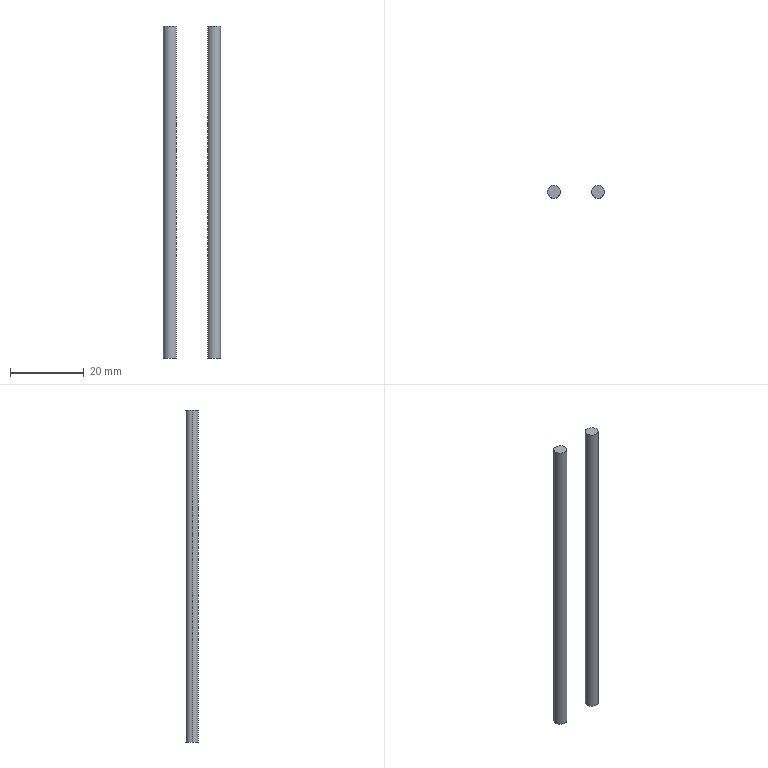Part | SolidWorks | features BaseBody 2 | 2 solids | 8 faces | box 15.5 x 3.5 x 90 mm | volume 1732 mm3 | plane 4 | cylinder 4 | commonest cylinder face diameters 3.5 x4
STEP:
#1=CARTESIAN_POINT('',(-1.75,0.,0.));
#2=VERTEX_POINT('',#1);
#3=CARTESIAN_POINT('',(1.75,0.,0.));
#4=VERTEX_POINT('',#3);
#5=CARTESIAN_POINT('',(0.,0.,0.));
#6=DIRECTION('',(0.,0.,1.));
#7=DIRECTION('',(1.,0.,0.));
#8=AXIS2_PLACEMENT_3D('',#5,#6,#7);
#9=CIRCLE('',#8,1.75);
#10=EDGE_CURVE('',#2,#4,#9,.T.);
#11=ORIENTED_EDGE('',*,*,#10,.F.);
#12=CARTESIAN_POINT('',(0.,0.,0.));
#13=DIRECTION('',(0.,0.,1.));
#14=DIRECTION('',(1.,0.,0.));
#15=AXIS2_PLACEMENT_3D('',#12,#13,#14);
#16=CIRCLE('',#15,1.75);
#17=EDGE_CURVE('',#4,#2,#16,.T.);
#18=ORIENTED_EDGE('',*,*,#17,.F.);
#19=EDGE_LOOP('',(#11,#18));
#20=FACE_OUTER_BOUND('',#19,.T.);
#21=CARTESIAN_POINT('',(0.,0.,0.));
#22=DIRECTION('',(0.,0.,1.));
#23=DIRECTION('',(1.,0.,0.));
#24=AXIS2_PLACEMENT_3D('',#21,#22,#23);
#25=PLANE('',#24);
#26=ADVANCED_FACE('',(#20),#25,.F.);
#27=CARTESIAN_POINT('',(-1.75,0.,90.));
#28=VERTEX_POINT('',#27);
#29=CARTESIAN_POINT('',(1.75,0.,90.));
#30=VERTEX_POINT('',#29);
#31=CARTESIAN_POINT('',(0.,0.,90.));
#32=DIRECTION('',(0.,0.,1.));
#33=DIRECTION('',(1.,0.,0.));
#34=AXIS2_PLACEMENT_3D('',#31,#32,#33);
#35=CIRCLE('',#34,1.75);
#36=EDGE_CURVE('',#28,#30,#35,.T.);
#37=ORIENTED_EDGE('',*,*,#36,.T.);
#38=CARTESIAN_POINT('',(0.,0.,90.));
#39=DIRECTION('',(0.,0.,1.));
#40=DIRECTION('',(1.,0.,0.));
#41=AXIS2_PLACEMENT_3D('',#38,#39,#40);
#42=CIRCLE('',#41,1.75);
#43=EDGE_CURVE('',#30,#28,#42,.T.);
#44=ORIENTED_EDGE('',*,*,#43,.T.);
#45=EDGE_LOOP('',(#37,#44));
#46=FACE_OUTER_BOUND('',#45,.T.);
#47=CARTESIAN_POINT('',(0.,0.,90.));
#48=DIRECTION('',(0.,0.,1.));
#49=DIRECTION('',(1.,0.,0.));
#50=AXIS2_PLACEMENT_3D('',#47,#48,#49);
#51=PLANE('',#50);
#52=ADVANCED_FACE('',(#46),#51,.T.);
#53=CARTESIAN_POINT('',(1.75,0.,90.));
#54=DIRECTION('',(0.,0.,-1.));
#55=VECTOR('',#54,1000.);
#56=LINE('',#53,#55);
#57=EDGE_CURVE('',#30,#4,#56,.T.);
#58=ORIENTED_EDGE('',*,*,#57,.F.);
#59=ORIENTED_EDGE('',*,*,#36,.F.);
#60=CARTESIAN_POINT('',(-1.75,0.,90.));
#61=DIRECTION('',(0.,0.,-1.));
#62=VECTOR('',#61,1000.);
#63=LINE('',#60,#62);
#64=EDGE_CURVE('',#28,#2,#63,.T.);
#65=ORIENTED_EDGE('',*,*,#64,.T.);
#66=ORIENTED_EDGE('',*,*,#10,.T.);
#67=EDGE_LOOP('',(#58,#59,#65,#66));
#68=FACE_OUTER_BOUND('',#67,.T.);
#69=CARTESIAN_POINT('',(0.,0.,90.));
#70=DIRECTION('',(0.,0.,-1.));
#71=DIRECTION('',(-1.,0.,0.));
#72=AXIS2_PLACEMENT_3D('',#69,#70,#71);
#73=CYLINDRICAL_SURFACE('',#72,1.75);
#74=ADVANCED_FACE('',(#68),#73,.T.);
#75=ORIENTED_EDGE('',*,*,#43,.F.);
#76=ORIENTED_EDGE('',*,*,#57,.T.);
#77=ORIENTED_EDGE('',*,*,#17,.T.);
#78=ORIENTED_EDGE('',*,*,#64,.F.);
#79=EDGE_LOOP('',(#75,#76,#77,#78));
#80=FACE_OUTER_BOUND('',#79,.T.);
#81=CARTESIAN_POINT('',(0.,0.,90.));
#82=DIRECTION('',(0.,0.,-1.));
#83=DIRECTION('',(-1.,0.,0.));
#84=AXIS2_PLACEMENT_3D('',#81,#82,#83);
#85=CYLINDRICAL_SURFACE('',#84,1.75);
#86=ADVANCED_FACE('',(#80),#85,.T.);
#87=CLOSED_SHELL('',(#26,#52,#74,#86));
#88=MANIFOLD_SOLID_BREP('',#87);
#89=CARTESIAN_POINT('',(10.25,0.,0.));
#90=VERTEX_POINT('',#89);
#91=CARTESIAN_POINT('',(13.75,0.,0.));
#92=VERTEX_POINT('',#91);
#93=CARTESIAN_POINT('',(12.,0.,0.));
#94=DIRECTION('',(0.,0.,1.));
#95=DIRECTION('',(1.,0.,0.));
#96=AXIS2_PLACEMENT_3D('',#93,#94,#95);
#97=CIRCLE('',#96,1.75);
#98=EDGE_CURVE('',#90,#92,#97,.T.);
#99=ORIENTED_EDGE('',*,*,#98,.F.);
#100=CARTESIAN_POINT('',(12.,0.,0.));
#101=DIRECTION('',(0.,0.,1.));
#102=DIRECTION('',(1.,0.,0.));
#103=AXIS2_PLACEMENT_3D('',#100,#101,#102);
#104=CIRCLE('',#103,1.75);
#105=EDGE_CURVE('',#92,#90,#104,.T.);
#106=ORIENTED_EDGE('',*,*,#105,.F.);
#107=EDGE_LOOP('',(#99,#106));
#108=FACE_OUTER_BOUND('',#107,.T.);
#109=CARTESIAN_POINT('',(12.,0.,0.));
#110=DIRECTION('',(0.,0.,1.));
#111=DIRECTION('',(1.,0.,0.));
#112=AXIS2_PLACEMENT_3D('',#109,#110,#111);
#113=PLANE('',#112);
#114=ADVANCED_FACE('',(#108),#113,.F.);
#115=CARTESIAN_POINT('',(10.25,0.,90.));
#116=VERTEX_POINT('',#115);
#117=CARTESIAN_POINT('',(13.75,0.,90.));
#118=VERTEX_POINT('',#117);
#119=CARTESIAN_POINT('',(12.,0.,90.));
#120=DIRECTION('',(0.,0.,1.));
#121=DIRECTION('',(1.,0.,0.));
#122=AXIS2_PLACEMENT_3D('',#119,#120,#121);
#123=CIRCLE('',#122,1.75);
#124=EDGE_CURVE('',#116,#118,#123,.T.);
#125=ORIENTED_EDGE('',*,*,#124,.T.);
#126=CARTESIAN_POINT('',(12.,0.,90.));
#127=DIRECTION('',(0.,0.,1.));
#128=DIRECTION('',(1.,0.,0.));
#129=AXIS2_PLACEMENT_3D('',#126,#127,#128);
#130=CIRCLE('',#129,1.75);
#131=EDGE_CURVE('',#118,#116,#130,.T.);
#132=ORIENTED_EDGE('',*,*,#131,.T.);
#133=EDGE_LOOP('',(#125,#132));
#134=FACE_OUTER_BOUND('',#133,.T.);
#135=CARTESIAN_POINT('',(12.,0.,90.));
#136=DIRECTION('',(0.,0.,1.));
#137=DIRECTION('',(1.,0.,0.));
#138=AXIS2_PLACEMENT_3D('',#135,#136,#137);
#139=PLANE('',#138);
#140=ADVANCED_FACE('',(#134),#139,.T.);
#141=CARTESIAN_POINT('',(13.75,0.,90.));
#142=DIRECTION('',(0.,0.,-1.));
#143=VECTOR('',#142,1000.);
#144=LINE('',#141,#143);
#145=EDGE_CURVE('',#118,#92,#144,.T.);
#146=ORIENTED_EDGE('',*,*,#145,.F.);
#147=ORIENTED_EDGE('',*,*,#124,.F.);
#148=CARTESIAN_POINT('',(10.25,0.,90.));
#149=DIRECTION('',(0.,0.,-1.));
#150=VECTOR('',#149,1000.);
#151=LINE('',#148,#150);
#152=EDGE_CURVE('',#116,#90,#151,.T.);
#153=ORIENTED_EDGE('',*,*,#152,.T.);
#154=ORIENTED_EDGE('',*,*,#98,.T.);
#155=EDGE_LOOP('',(#146,#147,#153,#154));
#156=FACE_OUTER_BOUND('',#155,.T.);
#157=CARTESIAN_POINT('',(12.,0.,90.));
#158=DIRECTION('',(0.,0.,-1.));
#159=DIRECTION('',(-1.,0.,0.));
#160=AXIS2_PLACEMENT_3D('',#157,#158,#159);
#161=CYLINDRICAL_SURFACE('',#160,1.75);
#162=ADVANCED_FACE('',(#156),#161,.T.);
#163=ORIENTED_EDGE('',*,*,#131,.F.);
#164=ORIENTED_EDGE('',*,*,#145,.T.);
#165=ORIENTED_EDGE('',*,*,#105,.T.);
#166=ORIENTED_EDGE('',*,*,#152,.F.);
#167=EDGE_LOOP('',(#163,#164,#165,#166));
#168=FACE_OUTER_BOUND('',#167,.T.);
#169=CARTESIAN_POINT('',(12.,0.,90.));
#170=DIRECTION('',(0.,0.,-1.));
#171=DIRECTION('',(-1.,0.,0.));
#172=AXIS2_PLACEMENT_3D('',#169,#170,#171);
#173=CYLINDRICAL_SURFACE('',#172,1.75);
#174=ADVANCED_FACE('',(#168),#173,.T.);
#175=CLOSED_SHELL('',(#114,#140,#162,#174));
#176=MANIFOLD_SOLID_BREP('',#175);
#177=CARTESIAN_POINT('',(0.,0.,0.));
#178=DIRECTION('',(0.,0.,1.));
#179=DIRECTION('',(1.,0.,0.));
#180=AXIS2_PLACEMENT_3D('',#177,#178,#179);
#181=(LENGTH_UNIT()NAMED_UNIT(*)SI_UNIT(.MILLI.,.METRE.));
#182=UNCERTAINTY_MEASURE_WITH_UNIT(LENGTH_MEASURE(0.00001),#181,'','');
#183=(NAMED_UNIT(*)PLANE_ANGLE_UNIT()SI_UNIT($,.RADIAN.));
#184=(NAMED_UNIT(*)SI_UNIT($,.STERADIAN.)SOLID_ANGLE_UNIT());
#185=(GEOMETRIC_REPRESENTATION_CONTEXT(3)GLOBAL_UNCERTAINTY_ASSIGNED_CONTEXT((#182))GLOBAL_UNIT_ASSIGNED_CONTEXT((#181,#183,#184))REPRESENTATION_CONTEXT('',''));
#186=ADVANCED_BREP_SHAPE_REPRESENTATION('',(#88,#176,#180),#185);